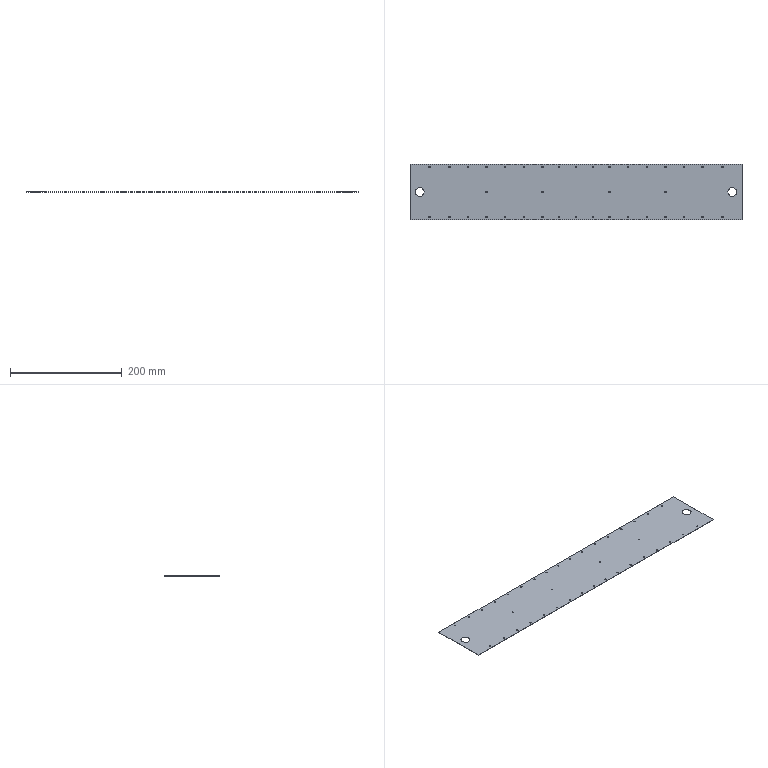Part | SolidWorks | features BaseBody 1 | 1 solid | 86 faces | box 594.4 x 100 x 0.5 mm | volume 29435 mm3 | cylinder 80 | plane 6 | commonest cylinder face diameters 2.4 x76 15.9 x4